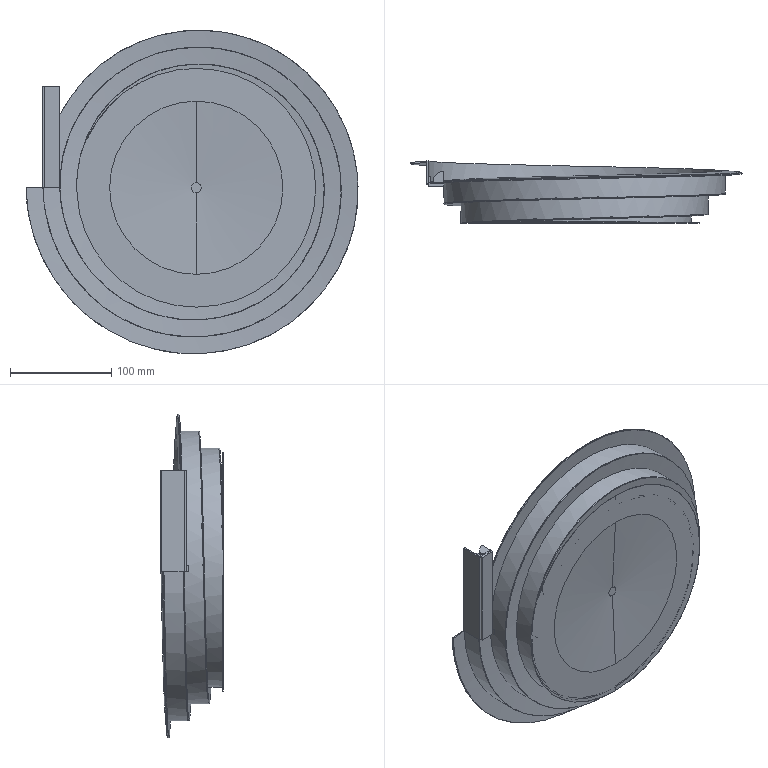Part | STEP file | X77a-01301 | 2 solids | 52 faces | box 328.723 x 61.502 x 320.354 mm | volume 216130 mm3 | plane 29 | spline 10 | cone 7 | cylinder 6 | commonest cylinder face diameters 236.378 x3 2.4 x2 4.6 x1